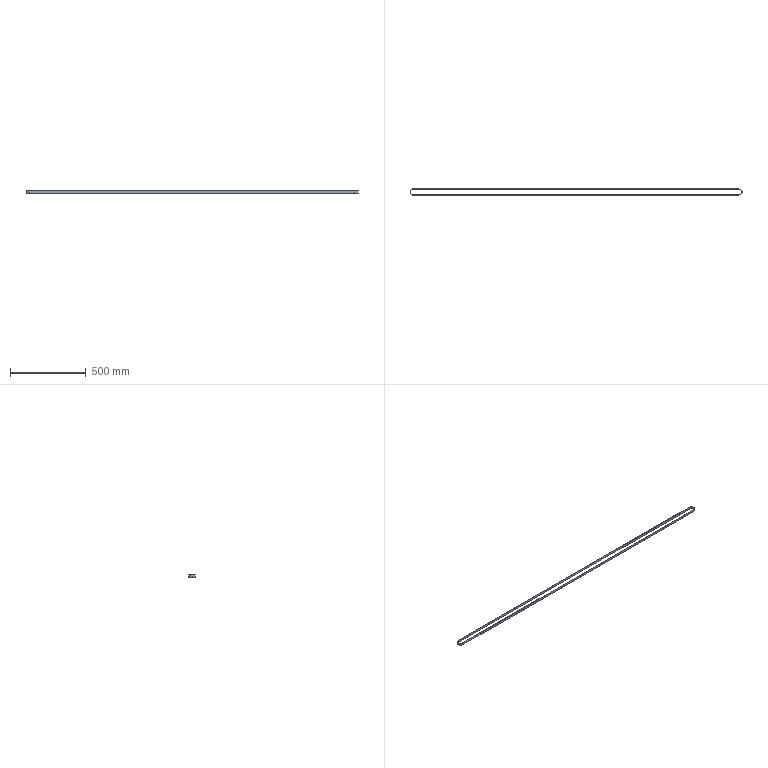Part | 1 solid | 12 faces | box 2196 x 40.83 x 15 mm | volume 66527 mm3 | cylinder 6 | plane 6 | commonest cylinder face diameters 38.83 x3 40.83 x3
STEP:
#1=CARTESIAN_POINT('',(0.,19.415,7.5));
#2=VERTEX_POINT('',#1);
#3=CARTESIAN_POINT('',(-19.415,0.,7.5));
#4=VERTEX_POINT('',#3);
#5=CARTESIAN_POINT('',(0.,0.,7.5));
#6=DIRECTION('',(0.,0.,1.));
#7=DIRECTION('',(-1.,0.,0.));
#8=AXIS2_PLACEMENT_3D('',#5,#6,#7);
#9=CIRCLE('',#8,19.415);
#10=EDGE_CURVE('',#2,#4,#9,.T.);
#11=ORIENTED_EDGE('',*,*,#10,.T.);
#12=CARTESIAN_POINT('',(-19.415,0.,-7.5));
#13=VERTEX_POINT('',#12);
#14=CARTESIAN_POINT('',(-19.415,0.,7.5));
#15=DIRECTION('',(0.,0.,-1.));
#16=VECTOR('',#15,1000.);
#17=LINE('',#14,#16);
#18=EDGE_CURVE('',#4,#13,#17,.T.);
#19=ORIENTED_EDGE('',*,*,#18,.T.);
#20=CARTESIAN_POINT('',(0.,19.415,-7.5));
#21=VERTEX_POINT('',#20);
#22=CARTESIAN_POINT('',(0.,0.,-7.5));
#23=DIRECTION('',(0.,0.,1.));
#24=DIRECTION('',(-1.,0.,0.));
#25=AXIS2_PLACEMENT_3D('',#22,#23,#24);
#26=CIRCLE('',#25,19.415);
#27=EDGE_CURVE('',#21,#13,#26,.T.);
#28=ORIENTED_EDGE('',*,*,#27,.F.);
#29=CARTESIAN_POINT('',(0.,19.415,7.5));
#30=DIRECTION('',(0.,0.,-1.));
#31=VECTOR('',#30,1000.);
#32=LINE('',#29,#31);
#33=EDGE_CURVE('',#2,#21,#32,.T.);
#34=ORIENTED_EDGE('',*,*,#33,.F.);
#35=EDGE_LOOP('',(#11,#19,#28,#34));
#36=FACE_OUTER_BOUND('',#35,.T.);
#37=CARTESIAN_POINT('',(0.,0.,7.5));
#38=DIRECTION('',(0.,0.,-1.));
#39=DIRECTION('',(-1.,0.,0.));
#40=AXIS2_PLACEMENT_3D('',#37,#38,#39);
#41=CYLINDRICAL_SURFACE('',#40,19.415);
#42=ADVANCED_FACE('',(#36),#41,.F.);
#43=CARTESIAN_POINT('',(-20.415,0.,7.5));
#44=VERTEX_POINT('',#43);
#45=CARTESIAN_POINT('',(0.,-20.415,7.5));
#46=VERTEX_POINT('',#45);
#47=CARTESIAN_POINT('',(0.,0.,7.5));
#48=DIRECTION('',(0.,0.,1.));
#49=DIRECTION('',(-1.,0.,0.));
#50=AXIS2_PLACEMENT_3D('',#47,#48,#49);
#51=CIRCLE('',#50,20.415);
#52=EDGE_CURVE('',#44,#46,#51,.T.);
#53=ORIENTED_EDGE('',*,*,#52,.F.);
#54=CARTESIAN_POINT('',(-20.415,0.,-7.5));
#55=VERTEX_POINT('',#54);
#56=CARTESIAN_POINT('',(-20.415,0.,7.5));
#57=DIRECTION('',(0.,0.,-1.));
#58=VECTOR('',#57,1000.);
#59=LINE('',#56,#58);
#60=EDGE_CURVE('',#44,#55,#59,.T.);
#61=ORIENTED_EDGE('',*,*,#60,.T.);
#62=CARTESIAN_POINT('',(0.,-20.415,-7.5));
#63=VERTEX_POINT('',#62);
#64=CARTESIAN_POINT('',(0.,0.,-7.5));
#65=DIRECTION('',(0.,0.,1.));
#66=DIRECTION('',(-1.,0.,0.));
#67=AXIS2_PLACEMENT_3D('',#64,#65,#66);
#68=CIRCLE('',#67,20.415);
#69=EDGE_CURVE('',#55,#63,#68,.T.);
#70=ORIENTED_EDGE('',*,*,#69,.T.);
#71=CARTESIAN_POINT('',(0.,-20.415,7.5));
#72=DIRECTION('',(0.,0.,-1.));
#73=VECTOR('',#72,1000.);
#74=LINE('',#71,#73);
#75=EDGE_CURVE('',#46,#63,#74,.T.);
#76=ORIENTED_EDGE('',*,*,#75,.F.);
#77=EDGE_LOOP('',(#53,#61,#70,#76));
#78=FACE_OUTER_BOUND('',#77,.T.);
#79=CARTESIAN_POINT('',(0.,0.,7.5));
#80=DIRECTION('',(0.,0.,-1.));
#81=DIRECTION('',(-1.,0.,0.));
#82=AXIS2_PLACEMENT_3D('',#79,#80,#81);
#83=CYLINDRICAL_SURFACE('',#82,20.415);
#84=ADVANCED_FACE('',(#78),#83,.T.);
#85=CARTESIAN_POINT('',(0.,20.415,7.5));
#86=VERTEX_POINT('',#85);
#87=CARTESIAN_POINT('',(0.,0.,7.5));
#88=DIRECTION('',(0.,0.,1.));
#89=DIRECTION('',(-1.,0.,0.));
#90=AXIS2_PLACEMENT_3D('',#87,#88,#89);
#91=CIRCLE('',#90,20.415);
#92=EDGE_CURVE('',#86,#44,#91,.T.);
#93=ORIENTED_EDGE('',*,*,#92,.T.);
#94=ORIENTED_EDGE('',*,*,#52,.T.);
#95=CARTESIAN_POINT('',(2155.,-20.415,7.5));
#96=VERTEX_POINT('',#95);
#97=CARTESIAN_POINT('',(0.,-20.415,7.5));
#98=DIRECTION('',(1.,0.,0.));
#99=VECTOR('',#98,1000.);
#100=LINE('',#97,#99);
#101=EDGE_CURVE('',#46,#96,#100,.T.);
#102=ORIENTED_EDGE('',*,*,#101,.T.);
#103=CARTESIAN_POINT('',(2155.,20.415,7.5));
#104=VERTEX_POINT('',#103);
#105=CARTESIAN_POINT('',(2155.,0.,7.5));
#106=DIRECTION('',(0.,0.,1.));
#107=DIRECTION('',(-1.,0.,0.));
#108=AXIS2_PLACEMENT_3D('',#105,#106,#107);
#109=CIRCLE('',#108,20.415);
#110=EDGE_CURVE('',#96,#104,#109,.T.);
#111=ORIENTED_EDGE('',*,*,#110,.T.);
#112=CARTESIAN_POINT('',(0.,20.415,7.5));
#113=DIRECTION('',(-1.,0.,0.));
#114=VECTOR('',#113,1000.);
#115=LINE('',#112,#114);
#116=EDGE_CURVE('',#104,#86,#115,.T.);
#117=ORIENTED_EDGE('',*,*,#116,.T.);
#118=EDGE_LOOP('',(#93,#94,#102,#111,#117));
#119=FACE_OUTER_BOUND('',#118,.T.);
#120=ORIENTED_EDGE('',*,*,#10,.F.);
#121=CARTESIAN_POINT('',(2155.,19.415,7.5));
#122=VERTEX_POINT('',#121);
#123=CARTESIAN_POINT('',(0.,19.415,7.5));
#124=DIRECTION('',(-1.,0.,0.));
#125=VECTOR('',#124,1000.);
#126=LINE('',#123,#125);
#127=EDGE_CURVE('',#122,#2,#126,.T.);
#128=ORIENTED_EDGE('',*,*,#127,.F.);
#129=CARTESIAN_POINT('',(2155.,-19.415,7.5));
#130=VERTEX_POINT('',#129);
#131=CARTESIAN_POINT('',(2155.,0.,7.5));
#132=DIRECTION('',(0.,0.,1.));
#133=DIRECTION('',(-1.,0.,0.));
#134=AXIS2_PLACEMENT_3D('',#131,#132,#133);
#135=CIRCLE('',#134,19.415);
#136=EDGE_CURVE('',#130,#122,#135,.T.);
#137=ORIENTED_EDGE('',*,*,#136,.F.);
#138=CARTESIAN_POINT('',(0.,-19.415,7.5));
#139=VERTEX_POINT('',#138);
#140=CARTESIAN_POINT('',(2155.,-19.415,7.5));
#141=DIRECTION('',(1.,0.,0.));
#142=VECTOR('',#141,1000.);
#143=LINE('',#140,#142);
#144=EDGE_CURVE('',#139,#130,#143,.T.);
#145=ORIENTED_EDGE('',*,*,#144,.F.);
#146=CARTESIAN_POINT('',(0.,0.,7.5));
#147=DIRECTION('',(0.,0.,1.));
#148=DIRECTION('',(-1.,0.,0.));
#149=AXIS2_PLACEMENT_3D('',#146,#147,#148);
#150=CIRCLE('',#149,19.415);
#151=EDGE_CURVE('',#4,#139,#150,.T.);
#152=ORIENTED_EDGE('',*,*,#151,.F.);
#153=EDGE_LOOP('',(#120,#128,#137,#145,#152));
#154=FACE_BOUND('',#153,.T.);
#155=CARTESIAN_POINT('',(0.,0.,7.5));
#156=DIRECTION('',(0.,0.,-1.));
#157=DIRECTION('',(-1.,0.,0.));
#158=AXIS2_PLACEMENT_3D('',#155,#156,#157);
#159=PLANE('',#158);
#160=ADVANCED_FACE('',(#119,#154),#159,.F.);
#161=CARTESIAN_POINT('',(0.,20.415,-7.5));
#162=VERTEX_POINT('',#161);
#163=CARTESIAN_POINT('',(0.,0.,-7.5));
#164=DIRECTION('',(0.,0.,1.));
#165=DIRECTION('',(-1.,0.,0.));
#166=AXIS2_PLACEMENT_3D('',#163,#164,#165);
#167=CIRCLE('',#166,20.415);
#168=EDGE_CURVE('',#162,#55,#167,.T.);
#169=ORIENTED_EDGE('',*,*,#168,.F.);
#170=CARTESIAN_POINT('',(2155.,20.415,-7.5));
#171=VERTEX_POINT('',#170);
#172=CARTESIAN_POINT('',(0.,20.415,-7.5));
#173=DIRECTION('',(-1.,0.,0.));
#174=VECTOR('',#173,1000.);
#175=LINE('',#172,#174);
#176=EDGE_CURVE('',#171,#162,#175,.T.);
#177=ORIENTED_EDGE('',*,*,#176,.F.);
#178=CARTESIAN_POINT('',(2155.,-20.415,-7.5));
#179=VERTEX_POINT('',#178);
#180=CARTESIAN_POINT('',(2155.,0.,-7.5));
#181=DIRECTION('',(0.,0.,1.));
#182=DIRECTION('',(-1.,0.,0.));
#183=AXIS2_PLACEMENT_3D('',#180,#181,#182);
#184=CIRCLE('',#183,20.415);
#185=EDGE_CURVE('',#179,#171,#184,.T.);
#186=ORIENTED_EDGE('',*,*,#185,.F.);
#187=CARTESIAN_POINT('',(0.,-20.415,-7.5));
#188=DIRECTION('',(1.,0.,0.));
#189=VECTOR('',#188,1000.);
#190=LINE('',#187,#189);
#191=EDGE_CURVE('',#63,#179,#190,.T.);
#192=ORIENTED_EDGE('',*,*,#191,.F.);
#193=ORIENTED_EDGE('',*,*,#69,.F.);
#194=EDGE_LOOP('',(#169,#177,#186,#192,#193));
#195=FACE_OUTER_BOUND('',#194,.T.);
#196=CARTESIAN_POINT('',(2155.,19.415,-7.5));
#197=VERTEX_POINT('',#196);
#198=CARTESIAN_POINT('',(0.,19.415,-7.5));
#199=DIRECTION('',(-1.,0.,0.));
#200=VECTOR('',#199,1000.);
#201=LINE('',#198,#200);
#202=EDGE_CURVE('',#197,#21,#201,.T.);
#203=ORIENTED_EDGE('',*,*,#202,.T.);
#204=ORIENTED_EDGE('',*,*,#27,.T.);
#205=CARTESIAN_POINT('',(0.,-19.415,-7.5));
#206=VERTEX_POINT('',#205);
#207=CARTESIAN_POINT('',(0.,0.,-7.5));
#208=DIRECTION('',(0.,0.,1.));
#209=DIRECTION('',(-1.,0.,0.));
#210=AXIS2_PLACEMENT_3D('',#207,#208,#209);
#211=CIRCLE('',#210,19.415);
#212=EDGE_CURVE('',#13,#206,#211,.T.);
#213=ORIENTED_EDGE('',*,*,#212,.T.);
#214=CARTESIAN_POINT('',(2155.,-19.415,-7.5));
#215=VERTEX_POINT('',#214);
#216=CARTESIAN_POINT('',(2155.,-19.415,-7.5));
#217=DIRECTION('',(1.,0.,0.));
#218=VECTOR('',#217,1000.);
#219=LINE('',#216,#218);
#220=EDGE_CURVE('',#206,#215,#219,.T.);
#221=ORIENTED_EDGE('',*,*,#220,.T.);
#222=CARTESIAN_POINT('',(2155.,0.,-7.5));
#223=DIRECTION('',(0.,0.,1.));
#224=DIRECTION('',(-1.,0.,0.));
#225=AXIS2_PLACEMENT_3D('',#222,#223,#224);
#226=CIRCLE('',#225,19.415);
#227=EDGE_CURVE('',#215,#197,#226,.T.);
#228=ORIENTED_EDGE('',*,*,#227,.T.);
#229=EDGE_LOOP('',(#203,#204,#213,#221,#228));
#230=FACE_BOUND('',#229,.T.);
#231=CARTESIAN_POINT('',(0.,0.,-7.5));
#232=DIRECTION('',(0.,0.,-1.));
#233=DIRECTION('',(-1.,0.,0.));
#234=AXIS2_PLACEMENT_3D('',#231,#232,#233);
#235=PLANE('',#234);
#236=ADVANCED_FACE('',(#195,#230),#235,.T.);
#237=ORIENTED_EDGE('',*,*,#60,.F.);
#238=ORIENTED_EDGE('',*,*,#92,.F.);
#239=CARTESIAN_POINT('',(0.,20.415,7.5));
#240=DIRECTION('',(0.,0.,-1.));
#241=VECTOR('',#240,1000.);
#242=LINE('',#239,#241);
#243=EDGE_CURVE('',#86,#162,#242,.T.);
#244=ORIENTED_EDGE('',*,*,#243,.T.);
#245=ORIENTED_EDGE('',*,*,#168,.T.);
#246=EDGE_LOOP('',(#237,#238,#244,#245));
#247=FACE_OUTER_BOUND('',#246,.T.);
#248=CARTESIAN_POINT('',(0.,0.,7.5));
#249=DIRECTION('',(0.,0.,-1.));
#250=DIRECTION('',(-1.,0.,0.));
#251=AXIS2_PLACEMENT_3D('',#248,#249,#250);
#252=CYLINDRICAL_SURFACE('',#251,20.415);
#253=ADVANCED_FACE('',(#247),#252,.T.);
#254=ORIENTED_EDGE('',*,*,#191,.T.);
#255=CARTESIAN_POINT('',(2155.,-20.415,7.5));
#256=DIRECTION('',(0.,0.,-1.));
#257=VECTOR('',#256,1000.);
#258=LINE('',#255,#257);
#259=EDGE_CURVE('',#96,#179,#258,.T.);
#260=ORIENTED_EDGE('',*,*,#259,.F.);
#261=ORIENTED_EDGE('',*,*,#101,.F.);
#262=ORIENTED_EDGE('',*,*,#75,.T.);
#263=EDGE_LOOP('',(#254,#260,#261,#262));
#264=FACE_OUTER_BOUND('',#263,.T.);
#265=CARTESIAN_POINT('',(0.,-20.415,7.5));
#266=DIRECTION('',(0.,1.,0.));
#267=DIRECTION('',(-1.,0.,0.));
#268=AXIS2_PLACEMENT_3D('',#265,#266,#267);
#269=PLANE('',#268);
#270=ADVANCED_FACE('',(#264),#269,.F.);
#271=ORIENTED_EDGE('',*,*,#185,.T.);
#272=CARTESIAN_POINT('',(2155.,20.415,7.5));
#273=DIRECTION('',(0.,0.,-1.));
#274=VECTOR('',#273,1000.);
#275=LINE('',#272,#274);
#276=EDGE_CURVE('',#104,#171,#275,.T.);
#277=ORIENTED_EDGE('',*,*,#276,.F.);
#278=ORIENTED_EDGE('',*,*,#110,.F.);
#279=ORIENTED_EDGE('',*,*,#259,.T.);
#280=EDGE_LOOP('',(#271,#277,#278,#279));
#281=FACE_OUTER_BOUND('',#280,.T.);
#282=CARTESIAN_POINT('',(2155.,0.,7.5));
#283=DIRECTION('',(0.,0.,-1.));
#284=DIRECTION('',(-1.,0.,0.));
#285=AXIS2_PLACEMENT_3D('',#282,#283,#284);
#286=CYLINDRICAL_SURFACE('',#285,20.415);
#287=ADVANCED_FACE('',(#281),#286,.T.);
#288=ORIENTED_EDGE('',*,*,#176,.T.);
#289=ORIENTED_EDGE('',*,*,#243,.F.);
#290=ORIENTED_EDGE('',*,*,#116,.F.);
#291=ORIENTED_EDGE('',*,*,#276,.T.);
#292=EDGE_LOOP('',(#288,#289,#290,#291));
#293=FACE_OUTER_BOUND('',#292,.T.);
#294=CARTESIAN_POINT('',(0.,20.415,7.5));
#295=DIRECTION('',(0.,-1.,0.));
#296=DIRECTION('',(1.,0.,0.));
#297=AXIS2_PLACEMENT_3D('',#294,#295,#296);
#298=PLANE('',#297);
#299=ADVANCED_FACE('',(#293),#298,.F.);
#300=ORIENTED_EDGE('',*,*,#18,.F.);
#301=ORIENTED_EDGE('',*,*,#151,.T.);
#302=CARTESIAN_POINT('',(0.,-19.415,7.5));
#303=DIRECTION('',(0.,0.,-1.));
#304=VECTOR('',#303,1000.);
#305=LINE('',#302,#304);
#306=EDGE_CURVE('',#139,#206,#305,.T.);
#307=ORIENTED_EDGE('',*,*,#306,.T.);
#308=ORIENTED_EDGE('',*,*,#212,.F.);
#309=EDGE_LOOP('',(#300,#301,#307,#308));
#310=FACE_OUTER_BOUND('',#309,.T.);
#311=CARTESIAN_POINT('',(0.,0.,7.5));
#312=DIRECTION('',(0.,0.,-1.));
#313=DIRECTION('',(-1.,0.,0.));
#314=AXIS2_PLACEMENT_3D('',#311,#312,#313);
#315=CYLINDRICAL_SURFACE('',#314,19.415);
#316=ADVANCED_FACE('',(#310),#315,.F.);
#317=ORIENTED_EDGE('',*,*,#220,.F.);
#318=ORIENTED_EDGE('',*,*,#306,.F.);
#319=ORIENTED_EDGE('',*,*,#144,.T.);
#320=CARTESIAN_POINT('',(2155.,-19.415,7.5));
#321=DIRECTION('',(0.,0.,-1.));
#322=VECTOR('',#321,1000.);
#323=LINE('',#320,#322);
#324=EDGE_CURVE('',#130,#215,#323,.T.);
#325=ORIENTED_EDGE('',*,*,#324,.T.);
#326=EDGE_LOOP('',(#317,#318,#319,#325));
#327=FACE_OUTER_BOUND('',#326,.T.);
#328=CARTESIAN_POINT('',(2155.,-19.415,7.5));
#329=DIRECTION('',(0.,1.,0.));
#330=DIRECTION('',(-1.,0.,0.));
#331=AXIS2_PLACEMENT_3D('',#328,#329,#330);
#332=PLANE('',#331);
#333=ADVANCED_FACE('',(#327),#332,.T.);
#334=ORIENTED_EDGE('',*,*,#227,.F.);
#335=ORIENTED_EDGE('',*,*,#324,.F.);
#336=ORIENTED_EDGE('',*,*,#136,.T.);
#337=CARTESIAN_POINT('',(2155.,19.415,7.5));
#338=DIRECTION('',(0.,0.,-1.));
#339=VECTOR('',#338,1000.);
#340=LINE('',#337,#339);
#341=EDGE_CURVE('',#122,#197,#340,.T.);
#342=ORIENTED_EDGE('',*,*,#341,.T.);
#343=EDGE_LOOP('',(#334,#335,#336,#342));
#344=FACE_OUTER_BOUND('',#343,.T.);
#345=CARTESIAN_POINT('',(2155.,0.,7.5));
#346=DIRECTION('',(0.,0.,-1.));
#347=DIRECTION('',(-1.,0.,0.));
#348=AXIS2_PLACEMENT_3D('',#345,#346,#347);
#349=CYLINDRICAL_SURFACE('',#348,19.415);
#350=ADVANCED_FACE('',(#344),#349,.F.);
#351=ORIENTED_EDGE('',*,*,#202,.F.);
#352=ORIENTED_EDGE('',*,*,#341,.F.);
#353=ORIENTED_EDGE('',*,*,#127,.T.);
#354=ORIENTED_EDGE('',*,*,#33,.T.);
#355=EDGE_LOOP('',(#351,#352,#353,#354));
#356=FACE_OUTER_BOUND('',#355,.T.);
#357=CARTESIAN_POINT('',(0.,19.415,7.5));
#358=DIRECTION('',(0.,-1.,0.));
#359=DIRECTION('',(1.,0.,0.));
#360=AXIS2_PLACEMENT_3D('',#357,#358,#359);
#361=PLANE('',#360);
#362=ADVANCED_FACE('',(#356),#361,.T.);
#363=CLOSED_SHELL('',(#42,#84,#160,#236,#253,#270,#287,#299,#316,#333,#350,#362));
#364=MANIFOLD_SOLID_BREP('',#363);
#365=CARTESIAN_POINT('',(0.,0.,0.));
#366=DIRECTION('',(0.,0.,1.));
#367=DIRECTION('',(1.,0.,0.));
#368=AXIS2_PLACEMENT_3D('',#365,#366,#367);
#369=(LENGTH_UNIT()NAMED_UNIT(*)SI_UNIT(.MILLI.,.METRE.));
#370=UNCERTAINTY_MEASURE_WITH_UNIT(LENGTH_MEASURE(0.00001),#369,'','');
#371=(NAMED_UNIT(*)PLANE_ANGLE_UNIT()SI_UNIT($,.RADIAN.));
#372=(NAMED_UNIT(*)SI_UNIT($,.STERADIAN.)SOLID_ANGLE_UNIT());
#373=(GEOMETRIC_REPRESENTATION_CONTEXT(3)GLOBAL_UNCERTAINTY_ASSIGNED_CONTEXT((#370))GLOBAL_UNIT_ASSIGNED_CONTEXT((#369,#371,#372))REPRESENTATION_CONTEXT('',''));
#374=ADVANCED_BREP_SHAPE_REPRESENTATION('',(#364,#368),#373);